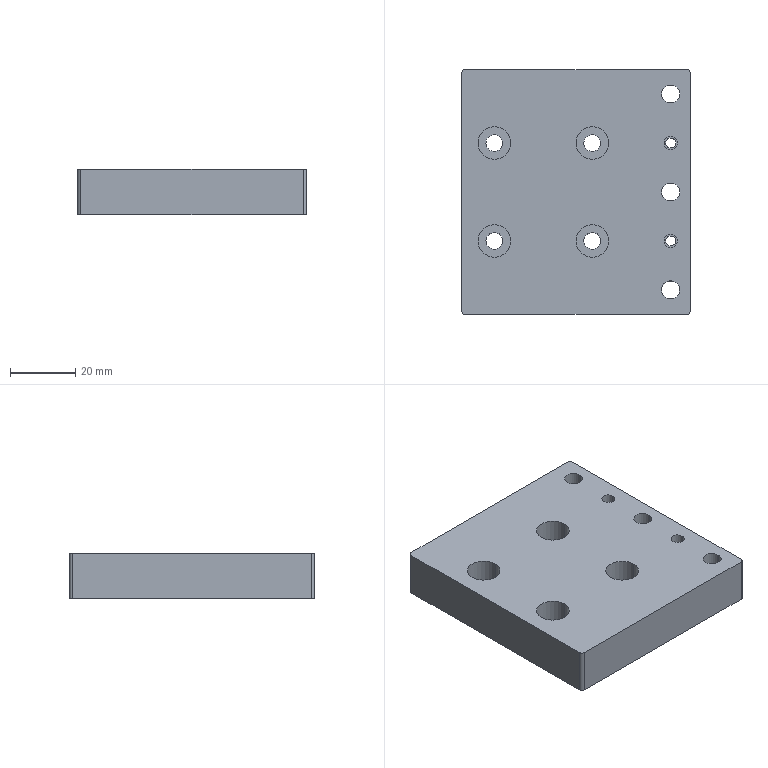Part | STEP file | 1 solid | 63 faces | box 70 x 75 x 14 mm | volume 67812 mm3 | cylinder 44 | plane 15 | cone 4 | commonest cylinder face diameters 10 x14 5.2 x8 5.5 x6 2 x4 2.5 x4 3 x4